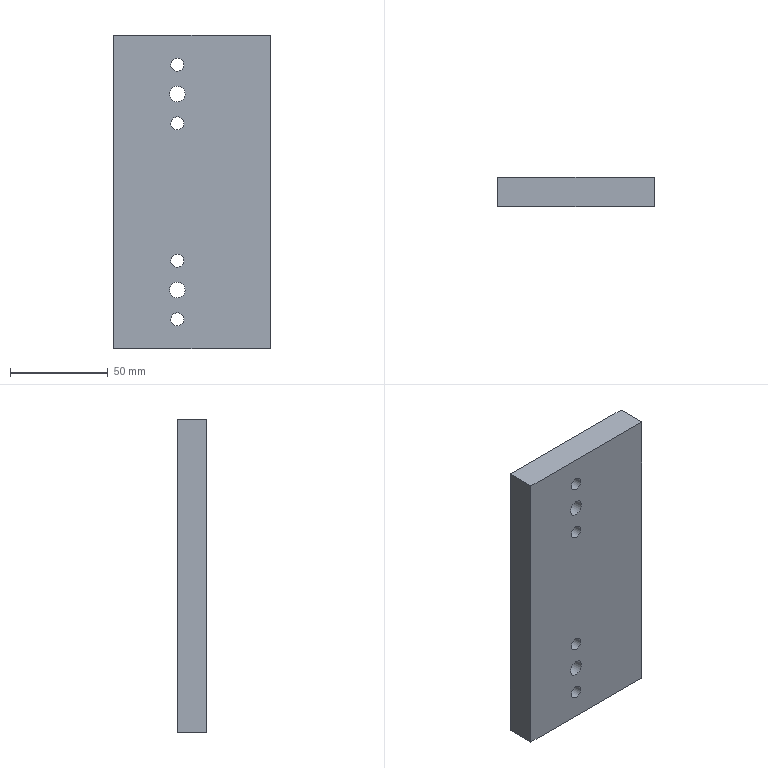Part | STEP file | SN10_008_006-03_PLACA | 1 solid | 12 faces | box 80 x 15 x 160 mm | volume 188410 mm3 | cylinder 6 | plane 6 | commonest cylinder face diameters 6.647 x4 8 x2
STEP:
#1=CARTESIAN_POINT('',(0.,0.,0.));
#2=DIRECTION('',(0.,0.,1.));
#3=DIRECTION('',(1.,0.,0.));
#4=AXIS2_PLACEMENT_3D('',#1,#2,#3);
#5=CARTESIAN_POINT('',(279.639,255.,304.352));
#6=VERTEX_POINT('',#5);
#7=CARTESIAN_POINT('',(276.129,255.,306.27));
#8=DIRECTION('',(0.,1.,0.));
#9=DIRECTION('',(1.,0.,0.));
#10=AXIS2_PLACEMENT_3D('',#7,#8,#9);
#11=CIRCLE('',#10,4.);
#12=CARTESIAN_POINT('',(276.129,255.1,306.27));
#13=DIRECTION('',(0.,1.,0.));
#14=DIRECTION('',(0.8776,0.,-0.4794));
#15=AXIS2_PLACEMENT_3D('',#12,#13,#14);
#16=CYLINDRICAL_SURFACE('',#15,4.);
#17=CARTESIAN_POINT('',(-0.5,-0.1));
#18=DIRECTION('',(1.,0.));
#19=VECTOR('',#18,1.);
#20=LINE('',#17,#19);
#21=(GEOMETRIC_REPRESENTATION_CONTEXT(2)PARAMETRIC_REPRESENTATION_CONTEXT()REPRESENTATION_CONTEXT('',''));
#22=DEFINITIONAL_REPRESENTATION('',(#20),#21);
#23=PCURVE('',#16,#22);
#24=CARTESIAN_POINT('',(0.,255.,0.));
#25=DIRECTION('',(0.,1.,0.));
#26=DIRECTION('',(0.,0.,1.));
#27=AXIS2_PLACEMENT_3D('',#24,#25,#26);
#28=PLANE('',#27);
#29=CARTESIAN_POINT('',(306.27,276.129));
#30=DIRECTION('',(0.,1.));
#31=AXIS2_PLACEMENT_2D('',#29,#30);
#32=CIRCLE('',#31,4.);
#33=(GEOMETRIC_REPRESENTATION_CONTEXT(2)PARAMETRIC_REPRESENTATION_CONTEXT()REPRESENTATION_CONTEXT('',''));
#34=DEFINITIONAL_REPRESENTATION('',(#32),#33);
#35=PCURVE('',#28,#34);
#36=SURFACE_CURVE('',#11,(#23,#35),.PCURVE_S1.);
#37=EDGE_CURVE('',#6,#6,#36,.T.);
#38=ORIENTED_EDGE('',*,*,#37,.T.);
#39=CARTESIAN_POINT('',(279.639,270.,304.352));
#40=VERTEX_POINT('',#39);
#41=CARTESIAN_POINT('',(279.639,255.,304.352));
#42=CARTESIAN_POINT('',(279.639,270.,304.352));
#43=B_SPLINE_CURVE_WITH_KNOTS('',1,(#41,#42),.UNSPECIFIED.,.F.,.F.,(2,2),(-0.1,14.9),.PIECEWISE_BEZIER_KNOTS.);
#44=CARTESIAN_POINT('',(6.283,0.));
#45=DIRECTION('',(0.,1.));
#46=VECTOR('',#45,1.);
#47=LINE('',#44,#46);
#48=(GEOMETRIC_REPRESENTATION_CONTEXT(2)PARAMETRIC_REPRESENTATION_CONTEXT()REPRESENTATION_CONTEXT('',''));
#49=DEFINITIONAL_REPRESENTATION('',(#47),#48);
#50=PCURVE('',#16,#49);
#51=CARTESIAN_POINT('',(0.,0.));
#52=DIRECTION('',(0.,1.));
#53=VECTOR('',#52,1.);
#54=LINE('',#51,#53);
#55=(GEOMETRIC_REPRESENTATION_CONTEXT(2)PARAMETRIC_REPRESENTATION_CONTEXT()REPRESENTATION_CONTEXT('',''));
#56=DEFINITIONAL_REPRESENTATION('',(#54),#55);
#57=PCURVE('',#16,#56);
#58=SEAM_CURVE('',#43,(#50,#57),.PCURVE_S1.);
#59=EDGE_CURVE('',#6,#40,#58,.T.);
#60=ORIENTED_EDGE('',*,*,#59,.T.);
#61=CARTESIAN_POINT('',(276.129,270.,306.27));
#62=DIRECTION('',(0.,1.,0.));
#63=DIRECTION('',(1.,0.,0.));
#64=AXIS2_PLACEMENT_3D('',#61,#62,#63);
#65=CIRCLE('',#64,4.);
#66=CARTESIAN_POINT('',(-0.5,14.9));
#67=DIRECTION('',(1.,0.));
#68=VECTOR('',#67,1.);
#69=LINE('',#66,#68);
#70=(GEOMETRIC_REPRESENTATION_CONTEXT(2)PARAMETRIC_REPRESENTATION_CONTEXT()REPRESENTATION_CONTEXT('',''));
#71=DEFINITIONAL_REPRESENTATION('',(#69),#70);
#72=PCURVE('',#16,#71);
#73=CARTESIAN_POINT('',(0.,270.,0.));
#74=DIRECTION('',(0.,1.,0.));
#75=DIRECTION('',(0.,0.,1.));
#76=AXIS2_PLACEMENT_3D('',#73,#74,#75);
#77=PLANE('',#76);
#78=CARTESIAN_POINT('',(306.27,276.129));
#79=DIRECTION('',(0.,1.));
#80=AXIS2_PLACEMENT_2D('',#78,#79);
#81=CIRCLE('',#80,4.);
#82=(GEOMETRIC_REPRESENTATION_CONTEXT(2)PARAMETRIC_REPRESENTATION_CONTEXT()REPRESENTATION_CONTEXT('',''));
#83=DEFINITIONAL_REPRESENTATION('',(#81),#82);
#84=PCURVE('',#77,#83);
#85=SURFACE_CURVE('',#65,(#72,#84),.PCURVE_S1.);
#86=EDGE_CURVE('',#40,#40,#85,.T.);
#87=ORIENTED_EDGE('',*,*,#86,.F.);
#88=ORIENTED_EDGE('',*,*,#59,.F.);
#89=EDGE_LOOP('',(#38,#60,#87,#88));
#90=FACE_BOUND('',#89,.F.);
#91=ADVANCED_FACE('',(#90),#16,.F.);
#92=CARTESIAN_POINT('',(323.629,270.,436.27));
#93=VERTEX_POINT('',#92);
#94=CARTESIAN_POINT('',(243.629,270.,436.27));
#95=VERTEX_POINT('',#94);
#96=CARTESIAN_POINT('',(323.629,270.,436.27));
#97=DIRECTION('',(-1.,0.,0.));
#98=VECTOR('',#97,1.);
#99=LINE('',#96,#98);
#100=CARTESIAN_POINT('',(436.27,323.629));
#101=DIRECTION('',(0.,-1.));
#102=VECTOR('',#101,1.);
#103=LINE('',#100,#102);
#104=(GEOMETRIC_REPRESENTATION_CONTEXT(2)PARAMETRIC_REPRESENTATION_CONTEXT()REPRESENTATION_CONTEXT('',''));
#105=DEFINITIONAL_REPRESENTATION('',(#103),#104);
#106=PCURVE('',#77,#105);
#107=CARTESIAN_POINT('',(323.629,270.,436.27));
#108=DIRECTION('',(0.,0.,1.));
#109=DIRECTION('',(1.,0.,0.));
#110=AXIS2_PLACEMENT_3D('',#107,#108,#109);
#111=PLANE('',#110);
#112=CARTESIAN_POINT('',(0.,0.));
#113=DIRECTION('',(-1.,0.));
#114=VECTOR('',#113,1.);
#115=LINE('',#112,#114);
#116=(GEOMETRIC_REPRESENTATION_CONTEXT(2)PARAMETRIC_REPRESENTATION_CONTEXT()REPRESENTATION_CONTEXT('',''));
#117=DEFINITIONAL_REPRESENTATION('',(#115),#116);
#118=PCURVE('',#111,#117);
#119=SURFACE_CURVE('',#99,(#106,#118),.PCURVE_S1.);
#120=EDGE_CURVE('',#93,#95,#119,.T.);
#121=ORIENTED_EDGE('',*,*,#120,.F.);
#122=CARTESIAN_POINT('',(323.629,270.,276.27));
#123=VERTEX_POINT('',#122);
#124=CARTESIAN_POINT('',(323.629,270.,276.27));
#125=DIRECTION('',(0.,0.,1.));
#126=VECTOR('',#125,1.);
#127=LINE('',#124,#126);
#128=CARTESIAN_POINT('',(276.27,323.629));
#129=DIRECTION('',(1.,0.));
#130=VECTOR('',#129,1.);
#131=LINE('',#128,#130);
#132=(GEOMETRIC_REPRESENTATION_CONTEXT(2)PARAMETRIC_REPRESENTATION_CONTEXT()REPRESENTATION_CONTEXT('',''));
#133=DEFINITIONAL_REPRESENTATION('',(#131),#132);
#134=PCURVE('',#77,#133);
#135=CARTESIAN_POINT('',(323.629,270.,276.27));
#136=DIRECTION('',(1.,0.,0.));
#137=DIRECTION('',(0.,0.,-1.));
#138=AXIS2_PLACEMENT_3D('',#135,#136,#137);
#139=PLANE('',#138);
#140=CARTESIAN_POINT('',(0.,0.));
#141=DIRECTION('',(-1.,0.));
#142=VECTOR('',#141,1.);
#143=LINE('',#140,#142);
#144=(GEOMETRIC_REPRESENTATION_CONTEXT(2)PARAMETRIC_REPRESENTATION_CONTEXT()REPRESENTATION_CONTEXT('',''));
#145=DEFINITIONAL_REPRESENTATION('',(#143),#144);
#146=PCURVE('',#139,#145);
#147=SURFACE_CURVE('',#127,(#134,#146),.PCURVE_S1.);
#148=EDGE_CURVE('',#123,#93,#147,.T.);
#149=ORIENTED_EDGE('',*,*,#148,.F.);
#150=CARTESIAN_POINT('',(243.629,270.,276.27));
#151=VERTEX_POINT('',#150);
#152=CARTESIAN_POINT('',(243.629,270.,276.27));
#153=DIRECTION('',(1.,0.,0.));
#154=VECTOR('',#153,1.);
#155=LINE('',#152,#154);
#156=CARTESIAN_POINT('',(276.27,243.629));
#157=DIRECTION('',(0.,1.));
#158=VECTOR('',#157,1.);
#159=LINE('',#156,#158);
#160=(GEOMETRIC_REPRESENTATION_CONTEXT(2)PARAMETRIC_REPRESENTATION_CONTEXT()REPRESENTATION_CONTEXT('',''));
#161=DEFINITIONAL_REPRESENTATION('',(#159),#160);
#162=PCURVE('',#77,#161);
#163=CARTESIAN_POINT('',(243.629,270.,276.27));
#164=DIRECTION('',(0.,0.,-1.));
#165=DIRECTION('',(-1.,0.,0.));
#166=AXIS2_PLACEMENT_3D('',#163,#164,#165);
#167=PLANE('',#166);
#168=CARTESIAN_POINT('',(0.,0.));
#169=DIRECTION('',(-1.,0.));
#170=VECTOR('',#169,1.);
#171=LINE('',#168,#170);
#172=(GEOMETRIC_REPRESENTATION_CONTEXT(2)PARAMETRIC_REPRESENTATION_CONTEXT()REPRESENTATION_CONTEXT('',''));
#173=DEFINITIONAL_REPRESENTATION('',(#171),#172);
#174=PCURVE('',#167,#173);
#175=SURFACE_CURVE('',#155,(#162,#174),.PCURVE_S1.);
#176=EDGE_CURVE('',#151,#123,#175,.T.);
#177=ORIENTED_EDGE('',*,*,#176,.F.);
#178=CARTESIAN_POINT('',(243.629,270.,436.27));
#179=DIRECTION('',(0.,0.,-1.));
#180=VECTOR('',#179,1.);
#181=LINE('',#178,#180);
#182=CARTESIAN_POINT('',(436.27,243.629));
#183=DIRECTION('',(-1.,0.));
#184=VECTOR('',#183,1.);
#185=LINE('',#182,#184);
#186=(GEOMETRIC_REPRESENTATION_CONTEXT(2)PARAMETRIC_REPRESENTATION_CONTEXT()REPRESENTATION_CONTEXT('',''));
#187=DEFINITIONAL_REPRESENTATION('',(#185),#186);
#188=PCURVE('',#77,#187);
#189=CARTESIAN_POINT('',(243.629,270.,436.27));
#190=DIRECTION('',(-1.,0.,0.));
#191=DIRECTION('',(0.,0.,1.));
#192=AXIS2_PLACEMENT_3D('',#189,#190,#191);
#193=PLANE('',#192);
#194=CARTESIAN_POINT('',(0.,0.));
#195=DIRECTION('',(-1.,0.));
#196=VECTOR('',#195,1.);
#197=LINE('',#194,#196);
#198=(GEOMETRIC_REPRESENTATION_CONTEXT(2)PARAMETRIC_REPRESENTATION_CONTEXT()REPRESENTATION_CONTEXT('',''));
#199=DEFINITIONAL_REPRESENTATION('',(#197),#198);
#200=PCURVE('',#193,#199);
#201=SURFACE_CURVE('',#181,(#188,#200),.PCURVE_S1.);
#202=EDGE_CURVE('',#95,#151,#201,.T.);
#203=ORIENTED_EDGE('',*,*,#202,.F.);
#204=EDGE_LOOP('',(#121,#149,#177,#203));
#205=FACE_BOUND('',#204,.T.);
#206=ORIENTED_EDGE('',*,*,#86,.F.);
#207=EDGE_LOOP('',(#206));
#208=FACE_BOUND('',#207,.T.);
#209=CARTESIAN_POINT('',(279.639,270.,404.352));
#210=VERTEX_POINT('',#209);
#211=CARTESIAN_POINT('',(276.129,270.,406.27));
#212=DIRECTION('',(0.,1.,0.));
#213=DIRECTION('',(1.,0.,0.));
#214=AXIS2_PLACEMENT_3D('',#211,#212,#213);
#215=CIRCLE('',#214,4.);
#216=CARTESIAN_POINT('',(406.27,276.129));
#217=DIRECTION('',(0.,1.));
#218=AXIS2_PLACEMENT_2D('',#216,#217);
#219=CIRCLE('',#218,4.);
#220=(GEOMETRIC_REPRESENTATION_CONTEXT(2)PARAMETRIC_REPRESENTATION_CONTEXT()REPRESENTATION_CONTEXT('',''));
#221=DEFINITIONAL_REPRESENTATION('',(#219),#220);
#222=PCURVE('',#77,#221);
#223=CARTESIAN_POINT('',(276.129,255.1,406.27));
#224=DIRECTION('',(0.,1.,0.));
#225=DIRECTION('',(0.8776,0.,-0.4794));
#226=AXIS2_PLACEMENT_3D('',#223,#224,#225);
#227=CYLINDRICAL_SURFACE('',#226,4.);
#228=CARTESIAN_POINT('',(-0.5,14.9));
#229=DIRECTION('',(1.,0.));
#230=VECTOR('',#229,1.);
#231=LINE('',#228,#230);
#232=(GEOMETRIC_REPRESENTATION_CONTEXT(2)PARAMETRIC_REPRESENTATION_CONTEXT()REPRESENTATION_CONTEXT('',''));
#233=DEFINITIONAL_REPRESENTATION('',(#231),#232);
#234=PCURVE('',#227,#233);
#235=SURFACE_CURVE('',#215,(#222,#234),.PCURVE_S1.);
#236=EDGE_CURVE('',#210,#210,#235,.T.);
#237=ORIENTED_EDGE('',*,*,#236,.F.);
#238=EDGE_LOOP('',(#237));
#239=FACE_BOUND('',#238,.T.);
#240=CARTESIAN_POINT('',(279.046,270.,289.677));
#241=VERTEX_POINT('',#240);
#242=CARTESIAN_POINT('',(276.129,270.,291.27));
#243=DIRECTION('',(0.,1.,0.));
#244=DIRECTION('',(1.,0.,0.));
#245=AXIS2_PLACEMENT_3D('',#242,#243,#244);
#246=CIRCLE('',#245,3.324);
#247=CARTESIAN_POINT('',(291.27,276.129));
#248=DIRECTION('',(0.,1.));
#249=AXIS2_PLACEMENT_2D('',#247,#248);
#250=CIRCLE('',#249,3.324);
#251=(GEOMETRIC_REPRESENTATION_CONTEXT(2)PARAMETRIC_REPRESENTATION_CONTEXT()REPRESENTATION_CONTEXT('',''));
#252=DEFINITIONAL_REPRESENTATION('',(#250),#251);
#253=PCURVE('',#77,#252);
#254=CARTESIAN_POINT('',(276.129,255.1,291.27));
#255=DIRECTION('',(0.,1.,0.));
#256=DIRECTION('',(0.8776,0.,-0.4794));
#257=AXIS2_PLACEMENT_3D('',#254,#255,#256);
#258=CYLINDRICAL_SURFACE('',#257,3.324);
#259=CARTESIAN_POINT('',(-0.5,14.9));
#260=DIRECTION('',(1.,0.));
#261=VECTOR('',#260,1.);
#262=LINE('',#259,#261);
#263=(GEOMETRIC_REPRESENTATION_CONTEXT(2)PARAMETRIC_REPRESENTATION_CONTEXT()REPRESENTATION_CONTEXT('',''));
#264=DEFINITIONAL_REPRESENTATION('',(#262),#263);
#265=PCURVE('',#258,#264);
#266=SURFACE_CURVE('',#246,(#253,#265),.PCURVE_S1.);
#267=EDGE_CURVE('',#241,#241,#266,.T.);
#268=ORIENTED_EDGE('',*,*,#267,.F.);
#269=EDGE_LOOP('',(#268));
#270=FACE_BOUND('',#269,.T.);
#271=CARTESIAN_POINT('',(279.046,270.,319.677));
#272=VERTEX_POINT('',#271);
#273=CARTESIAN_POINT('',(276.129,270.,321.27));
#274=DIRECTION('',(0.,1.,0.));
#275=DIRECTION('',(1.,0.,0.));
#276=AXIS2_PLACEMENT_3D('',#273,#274,#275);
#277=CIRCLE('',#276,3.324);
#278=CARTESIAN_POINT('',(321.27,276.129));
#279=DIRECTION('',(0.,1.));
#280=AXIS2_PLACEMENT_2D('',#278,#279);
#281=CIRCLE('',#280,3.324);
#282=(GEOMETRIC_REPRESENTATION_CONTEXT(2)PARAMETRIC_REPRESENTATION_CONTEXT()REPRESENTATION_CONTEXT('',''));
#283=DEFINITIONAL_REPRESENTATION('',(#281),#282);
#284=PCURVE('',#77,#283);
#285=CARTESIAN_POINT('',(276.129,255.1,321.27));
#286=DIRECTION('',(0.,1.,0.));
#287=DIRECTION('',(0.8776,0.,-0.4794));
#288=AXIS2_PLACEMENT_3D('',#285,#286,#287);
#289=CYLINDRICAL_SURFACE('',#288,3.324);
#290=CARTESIAN_POINT('',(-0.5,14.9));
#291=DIRECTION('',(1.,0.));
#292=VECTOR('',#291,1.);
#293=LINE('',#290,#292);
#294=(GEOMETRIC_REPRESENTATION_CONTEXT(2)PARAMETRIC_REPRESENTATION_CONTEXT()REPRESENTATION_CONTEXT('',''));
#295=DEFINITIONAL_REPRESENTATION('',(#293),#294);
#296=PCURVE('',#289,#295);
#297=SURFACE_CURVE('',#277,(#284,#296),.PCURVE_S1.);
#298=EDGE_CURVE('',#272,#272,#297,.T.);
#299=ORIENTED_EDGE('',*,*,#298,.F.);
#300=EDGE_LOOP('',(#299));
#301=FACE_BOUND('',#300,.T.);
#302=CARTESIAN_POINT('',(279.046,270.,389.677));
#303=VERTEX_POINT('',#302);
#304=CARTESIAN_POINT('',(276.129,270.,391.27));
#305=DIRECTION('',(0.,1.,0.));
#306=DIRECTION('',(1.,0.,0.));
#307=AXIS2_PLACEMENT_3D('',#304,#305,#306);
#308=CIRCLE('',#307,3.324);
#309=CARTESIAN_POINT('',(391.27,276.129));
#310=DIRECTION('',(0.,1.));
#311=AXIS2_PLACEMENT_2D('',#309,#310);
#312=CIRCLE('',#311,3.324);
#313=(GEOMETRIC_REPRESENTATION_CONTEXT(2)PARAMETRIC_REPRESENTATION_CONTEXT()REPRESENTATION_CONTEXT('',''));
#314=DEFINITIONAL_REPRESENTATION('',(#312),#313);
#315=PCURVE('',#77,#314);
#316=CARTESIAN_POINT('',(276.129,255.1,391.27));
#317=DIRECTION('',(0.,1.,0.));
#318=DIRECTION('',(0.8776,0.,-0.4794));
#319=AXIS2_PLACEMENT_3D('',#316,#317,#318);
#320=CYLINDRICAL_SURFACE('',#319,3.324);
#321=CARTESIAN_POINT('',(-0.5,14.9));
#322=DIRECTION('',(1.,0.));
#323=VECTOR('',#322,1.);
#324=LINE('',#321,#323);
#325=(GEOMETRIC_REPRESENTATION_CONTEXT(2)PARAMETRIC_REPRESENTATION_CONTEXT()REPRESENTATION_CONTEXT('',''));
#326=DEFINITIONAL_REPRESENTATION('',(#324),#325);
#327=PCURVE('',#320,#326);
#328=SURFACE_CURVE('',#308,(#315,#327),.PCURVE_S1.);
#329=EDGE_CURVE('',#303,#303,#328,.T.);
#330=ORIENTED_EDGE('',*,*,#329,.F.);
#331=EDGE_LOOP('',(#330));
#332=FACE_BOUND('',#331,.T.);
#333=CARTESIAN_POINT('',(279.046,270.,419.677));
#334=VERTEX_POINT('',#333);
#335=CARTESIAN_POINT('',(276.129,270.,421.27));
#336=DIRECTION('',(0.,1.,0.));
#337=DIRECTION('',(1.,0.,0.));
#338=AXIS2_PLACEMENT_3D('',#335,#336,#337);
#339=CIRCLE('',#338,3.324);
#340=CARTESIAN_POINT('',(421.27,276.129));
#341=DIRECTION('',(0.,1.));
#342=AXIS2_PLACEMENT_2D('',#340,#341);
#343=CIRCLE('',#342,3.324);
#344=(GEOMETRIC_REPRESENTATION_CONTEXT(2)PARAMETRIC_REPRESENTATION_CONTEXT()REPRESENTATION_CONTEXT('',''));
#345=DEFINITIONAL_REPRESENTATION('',(#343),#344);
#346=PCURVE('',#77,#345);
#347=CARTESIAN_POINT('',(276.129,255.1,421.27));
#348=DIRECTION('',(0.,1.,0.));
#349=DIRECTION('',(0.8776,0.,-0.4794));
#350=AXIS2_PLACEMENT_3D('',#347,#348,#349);
#351=CYLINDRICAL_SURFACE('',#350,3.324);
#352=CARTESIAN_POINT('',(-0.5,14.9));
#353=DIRECTION('',(1.,0.));
#354=VECTOR('',#353,1.);
#355=LINE('',#352,#354);
#356=(GEOMETRIC_REPRESENTATION_CONTEXT(2)PARAMETRIC_REPRESENTATION_CONTEXT()REPRESENTATION_CONTEXT('',''));
#357=DEFINITIONAL_REPRESENTATION('',(#355),#356);
#358=PCURVE('',#351,#357);
#359=SURFACE_CURVE('',#339,(#346,#358),.PCURVE_S1.);
#360=EDGE_CURVE('',#334,#334,#359,.T.);
#361=ORIENTED_EDGE('',*,*,#360,.F.);
#362=EDGE_LOOP('',(#361));
#363=FACE_BOUND('',#362,.T.);
#364=ADVANCED_FACE('',(#205,#208,#239,#270,#301,#332,#363),#77,.T.);
#365=CARTESIAN_POINT('',(323.629,255.,436.27));
#366=VERTEX_POINT('',#365);
#367=CARTESIAN_POINT('',(243.629,255.,436.27));
#368=VERTEX_POINT('',#367);
#369=CARTESIAN_POINT('',(323.629,255.,436.27));
#370=DIRECTION('',(-1.,0.,0.));
#371=VECTOR('',#370,1.);
#372=LINE('',#369,#371);
#373=CARTESIAN_POINT('',(0.,-15.));
#374=DIRECTION('',(-1.,0.));
#375=VECTOR('',#374,1.);
#376=LINE('',#373,#375);
#377=(GEOMETRIC_REPRESENTATION_CONTEXT(2)PARAMETRIC_REPRESENTATION_CONTEXT()REPRESENTATION_CONTEXT('',''));
#378=DEFINITIONAL_REPRESENTATION('',(#376),#377);
#379=PCURVE('',#111,#378);
#380=CARTESIAN_POINT('',(436.27,323.629));
#381=DIRECTION('',(0.,-1.));
#382=VECTOR('',#381,1.);
#383=LINE('',#380,#382);
#384=(GEOMETRIC_REPRESENTATION_CONTEXT(2)PARAMETRIC_REPRESENTATION_CONTEXT()REPRESENTATION_CONTEXT('',''));
#385=DEFINITIONAL_REPRESENTATION('',(#383),#384);
#386=PCURVE('',#28,#385);
#387=SURFACE_CURVE('',#372,(#379,#386),.PCURVE_S1.);
#388=EDGE_CURVE('',#366,#368,#387,.T.);
#389=ORIENTED_EDGE('',*,*,#388,.F.);
#390=CARTESIAN_POINT('',(323.629,270.,436.27));
#391=DIRECTION('',(0.,-1.,0.));
#392=VECTOR('',#391,1.);
#393=LINE('',#390,#392);
#394=CARTESIAN_POINT('',(0.,0.));
#395=DIRECTION('',(0.,-1.));
#396=VECTOR('',#395,1.);
#397=LINE('',#394,#396);
#398=(GEOMETRIC_REPRESENTATION_CONTEXT(2)PARAMETRIC_REPRESENTATION_CONTEXT()REPRESENTATION_CONTEXT('',''));
#399=DEFINITIONAL_REPRESENTATION('',(#397),#398);
#400=PCURVE('',#111,#399);
#401=CARTESIAN_POINT('',(-160.,0.));
#402=DIRECTION('',(0.,-1.));
#403=VECTOR('',#402,1.);
#404=LINE('',#401,#403);
#405=(GEOMETRIC_REPRESENTATION_CONTEXT(2)PARAMETRIC_REPRESENTATION_CONTEXT()REPRESENTATION_CONTEXT('',''));
#406=DEFINITIONAL_REPRESENTATION('',(#404),#405);
#407=PCURVE('',#139,#406);
#408=SURFACE_CURVE('',#393,(#400,#407),.PCURVE_S1.);
#409=EDGE_CURVE('',#93,#366,#408,.T.);
#410=ORIENTED_EDGE('',*,*,#409,.F.);
#411=ORIENTED_EDGE('',*,*,#120,.T.);
#412=CARTESIAN_POINT('',(243.629,270.,436.27));
#413=DIRECTION('',(0.,-1.,0.));
#414=VECTOR('',#413,1.);
#415=LINE('',#412,#414);
#416=CARTESIAN_POINT('',(-80.,0.));
#417=DIRECTION('',(0.,-1.));
#418=VECTOR('',#417,1.);
#419=LINE('',#416,#418);
#420=(GEOMETRIC_REPRESENTATION_CONTEXT(2)PARAMETRIC_REPRESENTATION_CONTEXT()REPRESENTATION_CONTEXT('',''));
#421=DEFINITIONAL_REPRESENTATION('',(#419),#420);
#422=PCURVE('',#111,#421);
#423=CARTESIAN_POINT('',(0.,0.));
#424=DIRECTION('',(0.,-1.));
#425=VECTOR('',#424,1.);
#426=LINE('',#423,#425);
#427=(GEOMETRIC_REPRESENTATION_CONTEXT(2)PARAMETRIC_REPRESENTATION_CONTEXT()REPRESENTATION_CONTEXT('',''));
#428=DEFINITIONAL_REPRESENTATION('',(#426),#427);
#429=PCURVE('',#193,#428);
#430=SURFACE_CURVE('',#415,(#422,#429),.PCURVE_S1.);
#431=EDGE_CURVE('',#95,#368,#430,.T.);
#432=ORIENTED_EDGE('',*,*,#431,.T.);
#433=EDGE_LOOP('',(#389,#410,#411,#432));
#434=FACE_BOUND('',#433,.T.);
#435=ADVANCED_FACE('',(#434),#111,.T.);
#436=CARTESIAN_POINT('',(323.629,255.,276.27));
#437=VERTEX_POINT('',#436);
#438=CARTESIAN_POINT('',(323.629,255.,276.27));
#439=DIRECTION('',(0.,0.,1.));
#440=VECTOR('',#439,1.);
#441=LINE('',#438,#440);
#442=CARTESIAN_POINT('',(0.,-15.));
#443=DIRECTION('',(-1.,0.));
#444=VECTOR('',#443,1.);
#445=LINE('',#442,#444);
#446=(GEOMETRIC_REPRESENTATION_CONTEXT(2)PARAMETRIC_REPRESENTATION_CONTEXT()REPRESENTATION_CONTEXT('',''));
#447=DEFINITIONAL_REPRESENTATION('',(#445),#446);
#448=PCURVE('',#139,#447);
#449=CARTESIAN_POINT('',(276.27,323.629));
#450=DIRECTION('',(1.,0.));
#451=VECTOR('',#450,1.);
#452=LINE('',#449,#451);
#453=(GEOMETRIC_REPRESENTATION_CONTEXT(2)PARAMETRIC_REPRESENTATION_CONTEXT()REPRESENTATION_CONTEXT('',''));
#454=DEFINITIONAL_REPRESENTATION('',(#452),#453);
#455=PCURVE('',#28,#454);
#456=SURFACE_CURVE('',#441,(#448,#455),.PCURVE_S1.);
#457=EDGE_CURVE('',#437,#366,#456,.T.);
#458=ORIENTED_EDGE('',*,*,#457,.F.);
#459=CARTESIAN_POINT('',(323.629,270.,276.27));
#460=DIRECTION('',(0.,-1.,0.));
#461=VECTOR('',#460,1.);
#462=LINE('',#459,#461);
#463=CARTESIAN_POINT('',(0.,0.));
#464=DIRECTION('',(0.,-1.));
#465=VECTOR('',#464,1.);
#466=LINE('',#463,#465);
#467=(GEOMETRIC_REPRESENTATION_CONTEXT(2)PARAMETRIC_REPRESENTATION_CONTEXT()REPRESENTATION_CONTEXT('',''));
#468=DEFINITIONAL_REPRESENTATION('',(#466),#467);
#469=PCURVE('',#139,#468);
#470=CARTESIAN_POINT('',(-80.,0.));
#471=DIRECTION('',(0.,-1.));
#472=VECTOR('',#471,1.);
#473=LINE('',#470,#472);
#474=(GEOMETRIC_REPRESENTATION_CONTEXT(2)PARAMETRIC_REPRESENTATION_CONTEXT()REPRESENTATION_CONTEXT('',''));
#475=DEFINITIONAL_REPRESENTATION('',(#473),#474);
#476=PCURVE('',#167,#475);
#477=SURFACE_CURVE('',#462,(#469,#476),.PCURVE_S1.);
#478=EDGE_CURVE('',#123,#437,#477,.T.);
#479=ORIENTED_EDGE('',*,*,#478,.F.);
#480=ORIENTED_EDGE('',*,*,#148,.T.);
#481=ORIENTED_EDGE('',*,*,#409,.T.);
#482=EDGE_LOOP('',(#458,#479,#480,#481));
#483=FACE_BOUND('',#482,.T.);
#484=ADVANCED_FACE('',(#483),#139,.T.);
#485=CARTESIAN_POINT('',(243.629,255.,276.27));
#486=VERTEX_POINT('',#485);
#487=CARTESIAN_POINT('',(243.629,255.,276.27));
#488=DIRECTION('',(1.,0.,0.));
#489=VECTOR('',#488,1.);
#490=LINE('',#487,#489);
#491=CARTESIAN_POINT('',(0.,-15.));
#492=DIRECTION('',(-1.,0.));
#493=VECTOR('',#492,1.);
#494=LINE('',#491,#493);
#495=(GEOMETRIC_REPRESENTATION_CONTEXT(2)PARAMETRIC_REPRESENTATION_CONTEXT()REPRESENTATION_CONTEXT('',''));
#496=DEFINITIONAL_REPRESENTATION('',(#494),#495);
#497=PCURVE('',#167,#496);
#498=CARTESIAN_POINT('',(276.27,243.629));
#499=DIRECTION('',(0.,1.));
#500=VECTOR('',#499,1.);
#501=LINE('',#498,#500);
#502=(GEOMETRIC_REPRESENTATION_CONTEXT(2)PARAMETRIC_REPRESENTATION_CONTEXT()REPRESENTATION_CONTEXT('',''));
#503=DEFINITIONAL_REPRESENTATION('',(#501),#502);
#504=PCURVE('',#28,#503);
#505=SURFACE_CURVE('',#490,(#497,#504),.PCURVE_S1.);
#506=EDGE_CURVE('',#486,#437,#505,.T.);
#507=ORIENTED_EDGE('',*,*,#506,.F.);
#508=CARTESIAN_POINT('',(243.629,270.,276.27));
#509=DIRECTION('',(0.,-1.,0.));
#510=VECTOR('',#509,1.);
#511=LINE('',#508,#510);
#512=CARTESIAN_POINT('',(0.,0.));
#513=DIRECTION('',(0.,-1.));
#514=VECTOR('',#513,1.);
#515=LINE('',#512,#514);
#516=(GEOMETRIC_REPRESENTATION_CONTEXT(2)PARAMETRIC_REPRESENTATION_CONTEXT()REPRESENTATION_CONTEXT('',''));
#517=DEFINITIONAL_REPRESENTATION('',(#515),#516);
#518=PCURVE('',#167,#517);
#519=CARTESIAN_POINT('',(-160.,0.));
#520=DIRECTION('',(0.,-1.));
#521=VECTOR('',#520,1.);
#522=LINE('',#519,#521);
#523=(GEOMETRIC_REPRESENTATION_CONTEXT(2)PARAMETRIC_REPRESENTATION_CONTEXT()REPRESENTATION_CONTEXT('',''));
#524=DEFINITIONAL_REPRESENTATION('',(#522),#523);
#525=PCURVE('',#193,#524);
#526=SURFACE_CURVE('',#511,(#518,#525),.PCURVE_S1.);
#527=EDGE_CURVE('',#151,#486,#526,.T.);
#528=ORIENTED_EDGE('',*,*,#527,.F.);
#529=ORIENTED_EDGE('',*,*,#176,.T.);
#530=ORIENTED_EDGE('',*,*,#478,.T.);
#531=EDGE_LOOP('',(#507,#528,#529,#530));
#532=FACE_BOUND('',#531,.T.);
#533=ADVANCED_FACE('',(#532),#167,.T.);
#534=CARTESIAN_POINT('',(243.629,255.,436.27));
#535=DIRECTION('',(0.,0.,-1.));
#536=VECTOR('',#535,1.);
#537=LINE('',#534,#536);
#538=CARTESIAN_POINT('',(0.,-15.));
#539=DIRECTION('',(-1.,0.));
#540=VECTOR('',#539,1.);
#541=LINE('',#538,#540);
#542=(GEOMETRIC_REPRESENTATION_CONTEXT(2)PARAMETRIC_REPRESENTATION_CONTEXT()REPRESENTATION_CONTEXT('',''));
#543=DEFINITIONAL_REPRESENTATION('',(#541),#542);
#544=PCURVE('',#193,#543);
#545=CARTESIAN_POINT('',(436.27,243.629));
#546=DIRECTION('',(-1.,0.));
#547=VECTOR('',#546,1.);
#548=LINE('',#545,#547);
#549=(GEOMETRIC_REPRESENTATION_CONTEXT(2)PARAMETRIC_REPRESENTATION_CONTEXT()REPRESENTATION_CONTEXT('',''));
#550=DEFINITIONAL_REPRESENTATION('',(#548),#549);
#551=PCURVE('',#28,#550);
#552=SURFACE_CURVE('',#537,(#544,#551),.PCURVE_S1.);
#553=EDGE_CURVE('',#368,#486,#552,.T.);
#554=ORIENTED_EDGE('',*,*,#553,.F.);
#555=ORIENTED_EDGE('',*,*,#431,.F.);
#556=ORIENTED_EDGE('',*,*,#202,.T.);
#557=ORIENTED_EDGE('',*,*,#527,.T.);
#558=EDGE_LOOP('',(#554,#555,#556,#557));
#559=FACE_BOUND('',#558,.T.);
#560=ADVANCED_FACE('',(#559),#193,.T.);
#561=CARTESIAN_POINT('',(279.046,255.,419.677));
#562=VERTEX_POINT('',#561);
#563=CARTESIAN_POINT('',(276.129,255.,421.27));
#564=DIRECTION('',(0.,1.,0.));
#565=DIRECTION('',(1.,0.,0.));
#566=AXIS2_PLACEMENT_3D('',#563,#564,#565);
#567=CIRCLE('',#566,3.324);
#568=CARTESIAN_POINT('',(-0.5,-0.1));
#569=DIRECTION('',(1.,0.));
#570=VECTOR('',#569,1.);
#571=LINE('',#568,#570);
#572=(GEOMETRIC_REPRESENTATION_CONTEXT(2)PARAMETRIC_REPRESENTATION_CONTEXT()REPRESENTATION_CONTEXT('',''));
#573=DEFINITIONAL_REPRESENTATION('',(#571),#572);
#574=PCURVE('',#351,#573);
#575=CARTESIAN_POINT('',(421.27,276.129));
#576=DIRECTION('',(0.,1.));
#577=AXIS2_PLACEMENT_2D('',#575,#576);
#578=CIRCLE('',#577,3.324);
#579=(GEOMETRIC_REPRESENTATION_CONTEXT(2)PARAMETRIC_REPRESENTATION_CONTEXT()REPRESENTATION_CONTEXT('',''));
#580=DEFINITIONAL_REPRESENTATION('',(#578),#579);
#581=PCURVE('',#28,#580);
#582=SURFACE_CURVE('',#567,(#574,#581),.PCURVE_S1.);
#583=EDGE_CURVE('',#562,#562,#582,.T.);
#584=ORIENTED_EDGE('',*,*,#583,.T.);
#585=CARTESIAN_POINT('',(279.046,255.,419.677));
#586=CARTESIAN_POINT('',(279.046,270.,419.677));
#587=B_SPLINE_CURVE_WITH_KNOTS('',1,(#585,#586),.UNSPECIFIED.,.F.,.F.,(2,2),(-0.1,14.9),.PIECEWISE_BEZIER_KNOTS.);
#588=CARTESIAN_POINT('',(6.283,0.));
#589=DIRECTION('',(0.,1.));
#590=VECTOR('',#589,1.);
#591=LINE('',#588,#590);
#592=(GEOMETRIC_REPRESENTATION_CONTEXT(2)PARAMETRIC_REPRESENTATION_CONTEXT()REPRESENTATION_CONTEXT('',''));
#593=DEFINITIONAL_REPRESENTATION('',(#591),#592);
#594=PCURVE('',#351,#593);
#595=CARTESIAN_POINT('',(0.,0.));
#596=DIRECTION('',(0.,1.));
#597=VECTOR('',#596,1.);
#598=LINE('',#595,#597);
#599=(GEOMETRIC_REPRESENTATION_CONTEXT(2)PARAMETRIC_REPRESENTATION_CONTEXT()REPRESENTATION_CONTEXT('',''));
#600=DEFINITIONAL_REPRESENTATION('',(#598),#599);
#601=PCURVE('',#351,#600);
#602=SEAM_CURVE('',#587,(#594,#601),.PCURVE_S1.);
#603=EDGE_CURVE('',#562,#334,#602,.T.);
#604=ORIENTED_EDGE('',*,*,#603,.T.);
#605=ORIENTED_EDGE('',*,*,#360,.F.);
#606=ORIENTED_EDGE('',*,*,#603,.F.);
#607=EDGE_LOOP('',(#584,#604,#605,#606));
#608=FACE_BOUND('',#607,.F.);
#609=ADVANCED_FACE('',(#608),#351,.F.);
#610=CARTESIAN_POINT('',(279.046,255.,389.677));
#611=VERTEX_POINT('',#610);
#612=CARTESIAN_POINT('',(276.129,255.,391.27));
#613=DIRECTION('',(0.,1.,0.));
#614=DIRECTION('',(1.,0.,0.));
#615=AXIS2_PLACEMENT_3D('',#612,#613,#614);
#616=CIRCLE('',#615,3.324);
#617=CARTESIAN_POINT('',(-0.5,-0.1));
#618=DIRECTION('',(1.,0.));
#619=VECTOR('',#618,1.);
#620=LINE('',#617,#619);
#621=(GEOMETRIC_REPRESENTATION_CONTEXT(2)PARAMETRIC_REPRESENTATION_CONTEXT()REPRESENTATION_CONTEXT('',''));
#622=DEFINITIONAL_REPRESENTATION('',(#620),#621);
#623=PCURVE('',#320,#622);
#624=CARTESIAN_POINT('',(391.27,276.129));
#625=DIRECTION('',(0.,1.));
#626=AXIS2_PLACEMENT_2D('',#624,#625);
#627=CIRCLE('',#626,3.324);
#628=(GEOMETRIC_REPRESENTATION_CONTEXT(2)PARAMETRIC_REPRESENTATION_CONTEXT()REPRESENTATION_CONTEXT('',''));
#629=DEFINITIONAL_REPRESENTATION('',(#627),#628);
#630=PCURVE('',#28,#629);
#631=SURFACE_CURVE('',#616,(#623,#630),.PCURVE_S1.);
#632=EDGE_CURVE('',#611,#611,#631,.T.);
#633=ORIENTED_EDGE('',*,*,#632,.T.);
#634=CARTESIAN_POINT('',(279.046,255.,389.677));
#635=CARTESIAN_POINT('',(279.046,270.,389.677));
#636=B_SPLINE_CURVE_WITH_KNOTS('',1,(#634,#635),.UNSPECIFIED.,.F.,.F.,(2,2),(-0.1,14.9),.PIECEWISE_BEZIER_KNOTS.);
#637=CARTESIAN_POINT('',(6.283,0.));
#638=DIRECTION('',(0.,1.));
#639=VECTOR('',#638,1.);
#640=LINE('',#637,#639);
#641=(GEOMETRIC_REPRESENTATION_CONTEXT(2)PARAMETRIC_REPRESENTATION_CONTEXT()REPRESENTATION_CONTEXT('',''));
#642=DEFINITIONAL_REPRESENTATION('',(#640),#641);
#643=PCURVE('',#320,#642);
#644=CARTESIAN_POINT('',(0.,0.));
#645=DIRECTION('',(0.,1.));
#646=VECTOR('',#645,1.);
#647=LINE('',#644,#646);
#648=(GEOMETRIC_REPRESENTATION_CONTEXT(2)PARAMETRIC_REPRESENTATION_CONTEXT()REPRESENTATION_CONTEXT('',''));
#649=DEFINITIONAL_REPRESENTATION('',(#647),#648);
#650=PCURVE('',#320,#649);
#651=SEAM_CURVE('',#636,(#643,#650),.PCURVE_S1.);
#652=EDGE_CURVE('',#611,#303,#651,.T.);
#653=ORIENTED_EDGE('',*,*,#652,.T.);
#654=ORIENTED_EDGE('',*,*,#329,.F.);
#655=ORIENTED_EDGE('',*,*,#652,.F.);
#656=EDGE_LOOP('',(#633,#653,#654,#655));
#657=FACE_BOUND('',#656,.F.);
#658=ADVANCED_FACE('',(#657),#320,.F.);
#659=CARTESIAN_POINT('',(279.046,255.,319.677));
#660=VERTEX_POINT('',#659);
#661=CARTESIAN_POINT('',(276.129,255.,321.27));
#662=DIRECTION('',(0.,1.,0.));
#663=DIRECTION('',(1.,0.,0.));
#664=AXIS2_PLACEMENT_3D('',#661,#662,#663);
#665=CIRCLE('',#664,3.324);
#666=CARTESIAN_POINT('',(-0.5,-0.1));
#667=DIRECTION('',(1.,0.));
#668=VECTOR('',#667,1.);
#669=LINE('',#666,#668);
#670=(GEOMETRIC_REPRESENTATION_CONTEXT(2)PARAMETRIC_REPRESENTATION_CONTEXT()REPRESENTATION_CONTEXT('',''));
#671=DEFINITIONAL_REPRESENTATION('',(#669),#670);
#672=PCURVE('',#289,#671);
#673=CARTESIAN_POINT('',(321.27,276.129));
#674=DIRECTION('',(0.,1.));
#675=AXIS2_PLACEMENT_2D('',#673,#674);
#676=CIRCLE('',#675,3.324);
#677=(GEOMETRIC_REPRESENTATION_CONTEXT(2)PARAMETRIC_REPRESENTATION_CONTEXT()REPRESENTATION_CONTEXT('',''));
#678=DEFINITIONAL_REPRESENTATION('',(#676),#677);
#679=PCURVE('',#28,#678);
#680=SURFACE_CURVE('',#665,(#672,#679),.PCURVE_S1.);
#681=EDGE_CURVE('',#660,#660,#680,.T.);
#682=ORIENTED_EDGE('',*,*,#681,.T.);
#683=CARTESIAN_POINT('',(279.046,255.,319.677));
#684=CARTESIAN_POINT('',(279.046,270.,319.677));
#685=B_SPLINE_CURVE_WITH_KNOTS('',1,(#683,#684),.UNSPECIFIED.,.F.,.F.,(2,2),(-0.1,14.9),.PIECEWISE_BEZIER_KNOTS.);
#686=CARTESIAN_POINT('',(6.283,0.));
#687=DIRECTION('',(0.,1.));
#688=VECTOR('',#687,1.);
#689=LINE('',#686,#688);
#690=(GEOMETRIC_REPRESENTATION_CONTEXT(2)PARAMETRIC_REPRESENTATION_CONTEXT()REPRESENTATION_CONTEXT('',''));
#691=DEFINITIONAL_REPRESENTATION('',(#689),#690);
#692=PCURVE('',#289,#691);
#693=CARTESIAN_POINT('',(0.,0.));
#694=DIRECTION('',(0.,1.));
#695=VECTOR('',#694,1.);
#696=LINE('',#693,#695);
#697=(GEOMETRIC_REPRESENTATION_CONTEXT(2)PARAMETRIC_REPRESENTATION_CONTEXT()REPRESENTATION_CONTEXT('',''));
#698=DEFINITIONAL_REPRESENTATION('',(#696),#697);
#699=PCURVE('',#289,#698);
#700=SEAM_CURVE('',#685,(#692,#699),.PCURVE_S1.);
#701=EDGE_CURVE('',#660,#272,#700,.T.);
#702=ORIENTED_EDGE('',*,*,#701,.T.);
#703=ORIENTED_EDGE('',*,*,#298,.F.);
#704=ORIENTED_EDGE('',*,*,#701,.F.);
#705=EDGE_LOOP('',(#682,#702,#703,#704));
#706=FACE_BOUND('',#705,.F.);
#707=ADVANCED_FACE('',(#706),#289,.F.);
#708=CARTESIAN_POINT('',(279.046,255.,289.677));
#709=VERTEX_POINT('',#708);
#710=CARTESIAN_POINT('',(276.129,255.,291.27));
#711=DIRECTION('',(0.,1.,0.));
#712=DIRECTION('',(1.,0.,0.));
#713=AXIS2_PLACEMENT_3D('',#710,#711,#712);
#714=CIRCLE('',#713,3.324);
#715=CARTESIAN_POINT('',(-0.5,-0.1));
#716=DIRECTION('',(1.,0.));
#717=VECTOR('',#716,1.);
#718=LINE('',#715,#717);
#719=(GEOMETRIC_REPRESENTATION_CONTEXT(2)PARAMETRIC_REPRESENTATION_CONTEXT()REPRESENTATION_CONTEXT('',''));
#720=DEFINITIONAL_REPRESENTATION('',(#718),#719);
#721=PCURVE('',#258,#720);
#722=CARTESIAN_POINT('',(291.27,276.129));
#723=DIRECTION('',(0.,1.));
#724=AXIS2_PLACEMENT_2D('',#722,#723);
#725=CIRCLE('',#724,3.324);
#726=(GEOMETRIC_REPRESENTATION_CONTEXT(2)PARAMETRIC_REPRESENTATION_CONTEXT()REPRESENTATION_CONTEXT('',''));
#727=DEFINITIONAL_REPRESENTATION('',(#725),#726);
#728=PCURVE('',#28,#727);
#729=SURFACE_CURVE('',#714,(#721,#728),.PCURVE_S1.);
#730=EDGE_CURVE('',#709,#709,#729,.T.);
#731=ORIENTED_EDGE('',*,*,#730,.T.);
#732=CARTESIAN_POINT('',(279.046,255.,289.677));
#733=CARTESIAN_POINT('',(279.046,270.,289.677));
#734=B_SPLINE_CURVE_WITH_KNOTS('',1,(#732,#733),.UNSPECIFIED.,.F.,.F.,(2,2),(-0.1,14.9),.PIECEWISE_BEZIER_KNOTS.);
#735=CARTESIAN_POINT('',(6.283,0.));
#736=DIRECTION('',(0.,1.));
#737=VECTOR('',#736,1.);
#738=LINE('',#735,#737);
#739=(GEOMETRIC_REPRESENTATION_CONTEXT(2)PARAMETRIC_REPRESENTATION_CONTEXT()REPRESENTATION_CONTEXT('',''));
#740=DEFINITIONAL_REPRESENTATION('',(#738),#739);
#741=PCURVE('',#258,#740);
#742=CARTESIAN_POINT('',(0.,0.));
#743=DIRECTION('',(0.,1.));
#744=VECTOR('',#743,1.);
#745=LINE('',#742,#744);
#746=(GEOMETRIC_REPRESENTATION_CONTEXT(2)PARAMETRIC_REPRESENTATION_CONTEXT()REPRESENTATION_CONTEXT('',''));
#747=DEFINITIONAL_REPRESENTATION('',(#745),#746);
#748=PCURVE('',#258,#747);
#749=SEAM_CURVE('',#734,(#741,#748),.PCURVE_S1.);
#750=EDGE_CURVE('',#709,#241,#749,.T.);
#751=ORIENTED_EDGE('',*,*,#750,.T.);
#752=ORIENTED_EDGE('',*,*,#267,.F.);
#753=ORIENTED_EDGE('',*,*,#750,.F.);
#754=EDGE_LOOP('',(#731,#751,#752,#753));
#755=FACE_BOUND('',#754,.F.);
#756=ADVANCED_FACE('',(#755),#258,.F.);
#757=CARTESIAN_POINT('',(279.639,255.,404.352));
#758=VERTEX_POINT('',#757);
#759=CARTESIAN_POINT('',(276.129,255.,406.27));
#760=DIRECTION('',(0.,1.,0.));
#761=DIRECTION('',(1.,0.,0.));
#762=AXIS2_PLACEMENT_3D('',#759,#760,#761);
#763=CIRCLE('',#762,4.);
#764=CARTESIAN_POINT('',(-0.5,-0.1));
#765=DIRECTION('',(1.,0.));
#766=VECTOR('',#765,1.);
#767=LINE('',#764,#766);
#768=(GEOMETRIC_REPRESENTATION_CONTEXT(2)PARAMETRIC_REPRESENTATION_CONTEXT()REPRESENTATION_CONTEXT('',''));
#769=DEFINITIONAL_REPRESENTATION('',(#767),#768);
#770=PCURVE('',#227,#769);
#771=CARTESIAN_POINT('',(406.27,276.129));
#772=DIRECTION('',(0.,1.));
#773=AXIS2_PLACEMENT_2D('',#771,#772);
#774=CIRCLE('',#773,4.);
#775=(GEOMETRIC_REPRESENTATION_CONTEXT(2)PARAMETRIC_REPRESENTATION_CONTEXT()REPRESENTATION_CONTEXT('',''));
#776=DEFINITIONAL_REPRESENTATION('',(#774),#775);
#777=PCURVE('',#28,#776);
#778=SURFACE_CURVE('',#763,(#770,#777),.PCURVE_S1.);
#779=EDGE_CURVE('',#758,#758,#778,.T.);
#780=ORIENTED_EDGE('',*,*,#779,.T.);
#781=CARTESIAN_POINT('',(279.639,255.,404.352));
#782=CARTESIAN_POINT('',(279.639,270.,404.352));
#783=B_SPLINE_CURVE_WITH_KNOTS('',1,(#781,#782),.UNSPECIFIED.,.F.,.F.,(2,2),(-0.1,14.9),.PIECEWISE_BEZIER_KNOTS.);
#784=CARTESIAN_POINT('',(6.283,0.));
#785=DIRECTION('',(0.,1.));
#786=VECTOR('',#785,1.);
#787=LINE('',#784,#786);
#788=(GEOMETRIC_REPRESENTATION_CONTEXT(2)PARAMETRIC_REPRESENTATION_CONTEXT()REPRESENTATION_CONTEXT('',''));
#789=DEFINITIONAL_REPRESENTATION('',(#787),#788);
#790=PCURVE('',#227,#789);
#791=CARTESIAN_POINT('',(0.,0.));
#792=DIRECTION('',(0.,1.));
#793=VECTOR('',#792,1.);
#794=LINE('',#791,#793);
#795=(GEOMETRIC_REPRESENTATION_CONTEXT(2)PARAMETRIC_REPRESENTATION_CONTEXT()REPRESENTATION_CONTEXT('',''));
#796=DEFINITIONAL_REPRESENTATION('',(#794),#795);
#797=PCURVE('',#227,#796);
#798=SEAM_CURVE('',#783,(#790,#797),.PCURVE_S1.);
#799=EDGE_CURVE('',#758,#210,#798,.T.);
#800=ORIENTED_EDGE('',*,*,#799,.T.);
#801=ORIENTED_EDGE('',*,*,#236,.F.);
#802=ORIENTED_EDGE('',*,*,#799,.F.);
#803=EDGE_LOOP('',(#780,#800,#801,#802));
#804=FACE_BOUND('',#803,.F.);
#805=ADVANCED_FACE('',(#804),#227,.F.);
#806=ORIENTED_EDGE('',*,*,#553,.T.);
#807=ORIENTED_EDGE('',*,*,#506,.T.);
#808=ORIENTED_EDGE('',*,*,#457,.T.);
#809=ORIENTED_EDGE('',*,*,#388,.T.);
#810=EDGE_LOOP('',(#806,#807,#808,#809));
#811=FACE_BOUND('',#810,.T.);
#812=ORIENTED_EDGE('',*,*,#37,.T.);
#813=EDGE_LOOP('',(#812));
#814=FACE_BOUND('',#813,.T.);
#815=ORIENTED_EDGE('',*,*,#779,.T.);
#816=EDGE_LOOP('',(#815));
#817=FACE_BOUND('',#816,.T.);
#818=ORIENTED_EDGE('',*,*,#730,.T.);
#819=EDGE_LOOP('',(#818));
#820=FACE_BOUND('',#819,.T.);
#821=ORIENTED_EDGE('',*,*,#681,.T.);
#822=EDGE_LOOP('',(#821));
#823=FACE_BOUND('',#822,.T.);
#824=ORIENTED_EDGE('',*,*,#632,.T.);
#825=EDGE_LOOP('',(#824));
#826=FACE_BOUND('',#825,.T.);
#827=ORIENTED_EDGE('',*,*,#583,.T.);
#828=EDGE_LOOP('',(#827));
#829=FACE_BOUND('',#828,.T.);
#830=ADVANCED_FACE('',(#811,#814,#817,#820,#823,#826,#829),#28,.F.);
#831=CLOSED_SHELL('',(#91,#364,#435,#484,#533,#560,#609,#658,#707,#756,#805,#830));
#832=MANIFOLD_SOLID_BREP('',#831);
#833=(LENGTH_UNIT()NAMED_UNIT(*)SI_UNIT(.MILLI.,.METRE.));
#834=UNCERTAINTY_MEASURE_WITH_UNIT(LENGTH_MEASURE(0.000005),#833,'','');
#835=(NAMED_UNIT(*)PLANE_ANGLE_UNIT()SI_UNIT($,.RADIAN.));
#836=(NAMED_UNIT(*)SI_UNIT($,.STERADIAN.)SOLID_ANGLE_UNIT());
#837=(GEOMETRIC_REPRESENTATION_CONTEXT(3)GLOBAL_UNCERTAINTY_ASSIGNED_CONTEXT((#834))GLOBAL_UNIT_ASSIGNED_CONTEXT((#833,#835,#836))REPRESENTATION_CONTEXT('',''));
#838=ADVANCED_BREP_SHAPE_REPRESENTATION('',(#4,#832),#837);